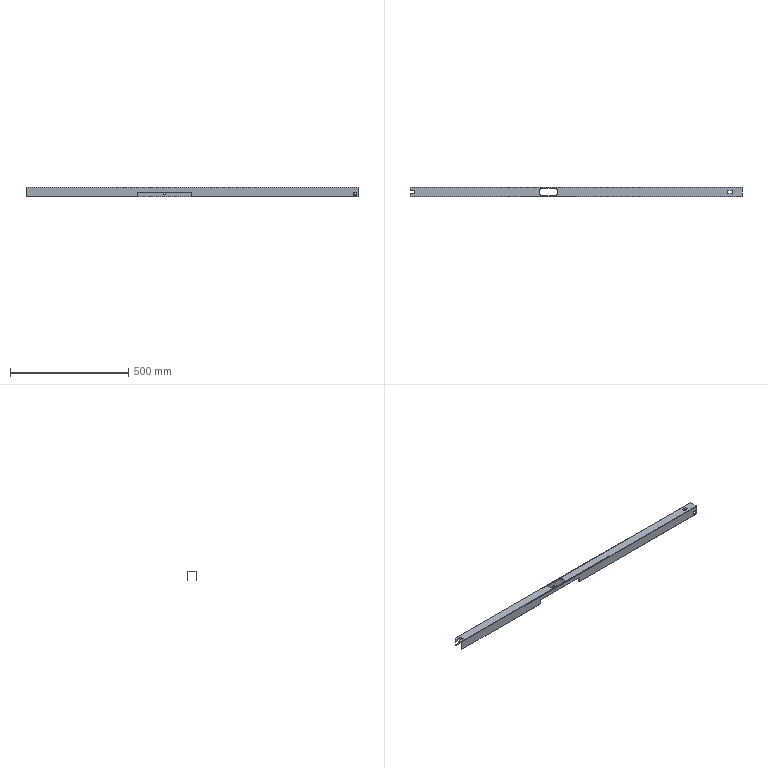Part | SolidWorks | features Cut 4, ICE 2, SMBaseFlange 2, FlatPattern 1, SheetMetal 1 | 1 solid | 68 faces | box 1402 x 38 x 40 mm | volume 225923 mm3 | plane 48 | cylinder 20 | commonest cylinder face diameters 10 x10 0.4 x2 3.4 x2 11 x2 15 x2 30 x2